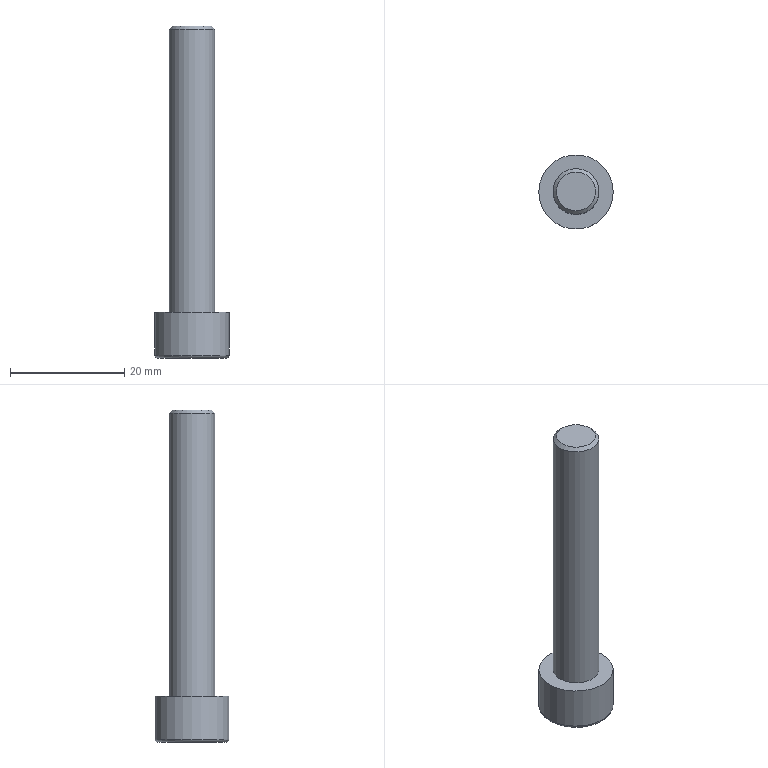Part | STEP file | 200 mesh_id82_xmt | 1 solid | 20 faces | box 13 x 13 x 58 mm | volume 3412 mm3 | plane 10 | cylinder 8 | torus 1 | cone 1 | commonest cylinder face diameters 0.6 x6 8 x1 13 x1
STEP:
#1=CARTESIAN_POINT('',(-17011.184,-4112.174,94.258));
#2=VERTEX_POINT('',#1);
#3=CARTESIAN_POINT('',(-17007.884,-4114.08,94.258));
#4=VERTEX_POINT('',#3);
#5=CARTESIAN_POINT('',(-17009.534,-4113.127,94.258));
#6=DIRECTION('',(0.866,-0.5,0.));
#7=VECTOR('',#6,1.);
#8=LINE('',#5,#7);
#9=EDGE_CURVE('',#2,#4,#8,.T.);
#10=ORIENTED_EDGE('',*,*,#9,.T.);
#11=CARTESIAN_POINT('',(-17004.584,-4112.174,94.258));
#12=VERTEX_POINT('',#11);
#13=CARTESIAN_POINT('',(-17006.234,-4113.127,94.258));
#14=DIRECTION('',(0.866,0.5,0.));
#15=VECTOR('',#14,1.);
#16=LINE('',#13,#15);
#17=EDGE_CURVE('',#4,#12,#16,.T.);
#18=ORIENTED_EDGE('',*,*,#17,.T.);
#19=CARTESIAN_POINT('',(-17004.584,-4108.364,94.258));
#20=VERTEX_POINT('',#19);
#21=CARTESIAN_POINT('',(-17004.584,-4110.269,94.258));
#22=DIRECTION('',(0.,1.,0.));
#23=VECTOR('',#22,1.);
#24=LINE('',#21,#23);
#25=EDGE_CURVE('',#12,#20,#24,.T.);
#26=ORIENTED_EDGE('',*,*,#25,.T.);
#27=CARTESIAN_POINT('',(-17007.884,-4106.459,94.258));
#28=VERTEX_POINT('',#27);
#29=CARTESIAN_POINT('',(-17006.234,-4107.411,94.258));
#30=DIRECTION('',(-0.866,0.5,0.));
#31=VECTOR('',#30,1.);
#32=LINE('',#29,#31);
#33=EDGE_CURVE('',#20,#28,#32,.T.);
#34=ORIENTED_EDGE('',*,*,#33,.T.);
#35=CARTESIAN_POINT('',(-17011.184,-4108.364,94.258));
#36=VERTEX_POINT('',#35);
#37=CARTESIAN_POINT('',(-17009.534,-4107.411,94.258));
#38=DIRECTION('',(-0.866,-0.5,0.));
#39=VECTOR('',#38,1.);
#40=LINE('',#37,#39);
#41=EDGE_CURVE('',#28,#36,#40,.T.);
#42=ORIENTED_EDGE('',*,*,#41,.T.);
#43=CARTESIAN_POINT('',(-17011.184,-4110.269,94.258));
#44=DIRECTION('',(0.,-1.,0.));
#45=VECTOR('',#44,1.);
#46=LINE('',#43,#45);
#47=EDGE_CURVE('',#36,#2,#46,.T.);
#48=ORIENTED_EDGE('',*,*,#47,.T.);
#49=EDGE_LOOP('',(#10,#18,#26,#34,#42,#48));
#50=FACE_BOUND('',#49,.T.);
#51=CARTESIAN_POINT('',(-17013.884,-4110.269,94.258));
#52=VERTEX_POINT('',#51);
#53=CARTESIAN_POINT('',(-17007.884,-4110.269,94.258));
#54=DIRECTION('',(0.,0.,-1.));
#55=DIRECTION('',(-1.,0.,0.));
#56=AXIS2_PLACEMENT_3D('',#53,#54,#55);
#57=CIRCLE('',#56,6.);
#58=EDGE_CURVE('',#52,#52,#57,.T.);
#59=ORIENTED_EDGE('',*,*,#58,.T.);
#60=EDGE_LOOP('',(#59));
#61=FACE_BOUND('',#60,.T.);
#62=CARTESIAN_POINT('',(-17007.884,-4110.269,94.258));
#63=DIRECTION('',(0.,0.,-1.));
#64=DIRECTION('',(-1.,0.,0.));
#65=AXIS2_PLACEMENT_3D('',#62,#63,#64);
#66=PLANE('',#65);
#67=ADVANCED_FACE('',(#50,#61),#66,.T.);
#68=CARTESIAN_POINT('',(-17003.884,-4110.269,151.658));
#69=VERTEX_POINT('',#68);
#70=CARTESIAN_POINT('',(-17007.884,-4110.269,151.658));
#71=DIRECTION('',(0.,0.,-1.));
#72=DIRECTION('',(1.,0.,0.));
#73=AXIS2_PLACEMENT_3D('',#70,#71,#72);
#74=CIRCLE('',#73,4.);
#75=EDGE_CURVE('',#69,#69,#74,.T.);
#76=ORIENTED_EDGE('',*,*,#75,.T.);
#77=EDGE_LOOP('',(#76));
#78=FACE_BOUND('',#77,.T.);
#79=CARTESIAN_POINT('',(-17003.884,-4110.269,102.258));
#80=VERTEX_POINT('',#79);
#81=CARTESIAN_POINT('',(-17007.884,-4110.269,102.258));
#82=DIRECTION('',(0.,0.,-1.));
#83=DIRECTION('',(1.,0.,0.));
#84=AXIS2_PLACEMENT_3D('',#81,#82,#83);
#85=CIRCLE('',#84,4.);
#86=EDGE_CURVE('',#80,#80,#85,.T.);
#87=ORIENTED_EDGE('',*,*,#86,.F.);
#88=EDGE_LOOP('',(#87));
#89=FACE_BOUND('',#88,.T.);
#90=CARTESIAN_POINT('',(-17007.884,-4110.269,102.258));
#91=DIRECTION('',(0.,0.,1.));
#92=DIRECTION('',(1.,0.,0.));
#93=AXIS2_PLACEMENT_3D('',#90,#91,#92);
#94=CYLINDRICAL_SURFACE('',#93,4.);
#95=ADVANCED_FACE('',(#78,#89),#94,.T.);
#96=ORIENTED_EDGE('',*,*,#86,.T.);
#97=EDGE_LOOP('',(#96));
#98=FACE_BOUND('',#97,.T.);
#99=CARTESIAN_POINT('',(-17001.384,-4110.269,102.258));
#100=VERTEX_POINT('',#99);
#101=CARTESIAN_POINT('',(-17007.884,-4110.269,102.258));
#102=DIRECTION('',(0.,0.,-1.));
#103=DIRECTION('',(1.,0.,0.));
#104=AXIS2_PLACEMENT_3D('',#101,#102,#103);
#105=CIRCLE('',#104,6.5);
#106=EDGE_CURVE('',#100,#100,#105,.T.);
#107=ORIENTED_EDGE('',*,*,#106,.F.);
#108=EDGE_LOOP('',(#107));
#109=FACE_BOUND('',#108,.T.);
#110=CARTESIAN_POINT('',(-17007.884,-4110.269,102.258));
#111=DIRECTION('',(0.,0.,1.));
#112=DIRECTION('',(1.,0.,0.));
#113=AXIS2_PLACEMENT_3D('',#110,#111,#112);
#114=PLANE('',#113);
#115=ADVANCED_FACE('',(#98,#109),#114,.T.);
#116=CARTESIAN_POINT('',(-17014.384,-4110.269,94.758));
#117=VERTEX_POINT('',#116);
#118=CARTESIAN_POINT('',(-17007.884,-4110.269,94.758));
#119=DIRECTION('',(0.,0.,1.));
#120=DIRECTION('',(-1.,0.,0.));
#121=AXIS2_PLACEMENT_3D('',#118,#119,#120);
#122=CIRCLE('',#121,6.5);
#123=EDGE_CURVE('',#117,#117,#122,.T.);
#124=ORIENTED_EDGE('',*,*,#123,.T.);
#125=EDGE_LOOP('',(#124));
#126=FACE_BOUND('',#125,.T.);
#127=ORIENTED_EDGE('',*,*,#106,.T.);
#128=EDGE_LOOP('',(#127));
#129=FACE_BOUND('',#128,.T.);
#130=CARTESIAN_POINT('',(-17007.884,-4110.269,102.258));
#131=DIRECTION('',(0.,0.,-1.));
#132=DIRECTION('',(1.,0.,0.));
#133=AXIS2_PLACEMENT_3D('',#130,#131,#132);
#134=CYLINDRICAL_SURFACE('',#133,6.5);
#135=ADVANCED_FACE('',(#126,#129),#134,.T.);
#136=ORIENTED_EDGE('',*,*,#58,.F.);
#137=EDGE_LOOP('',(#136));
#138=FACE_BOUND('',#137,.T.);
#139=ORIENTED_EDGE('',*,*,#123,.F.);
#140=EDGE_LOOP('',(#139));
#141=FACE_BOUND('',#140,.T.);
#142=CARTESIAN_POINT('',(-17007.884,-4110.269,94.758));
#143=DIRECTION('',(0.,0.,-1.));
#144=DIRECTION('',(-1.,0.,0.));
#145=AXIS2_PLACEMENT_3D('',#142,#143,#144);
#146=TOROIDAL_SURFACE('',#145,6.,0.5);
#147=ADVANCED_FACE('',(#138,#141),#146,.T.);
#148=CARTESIAN_POINT('',(-17007.884,-4113.733,94.558));
#149=VERTEX_POINT('',#148);
#150=CARTESIAN_POINT('',(-17007.884,-4113.733,99.258));
#151=VERTEX_POINT('',#150);
#152=CARTESIAN_POINT('',(-17007.884,-4113.733,99.258));
#153=DIRECTION('',(0.,0.,1.));
#154=VECTOR('',#153,1.);
#155=LINE('',#152,#154);
#156=EDGE_CURVE('',#149,#151,#155,.T.);
#157=ORIENTED_EDGE('',*,*,#156,.F.);
#158=CARTESIAN_POINT('',(-17010.884,-4112.001,94.558));
#159=VERTEX_POINT('',#158);
#160=CARTESIAN_POINT('',(-17010.884,-4112.001,94.558));
#161=DIRECTION('',(-0.866,0.5,0.));
#162=VECTOR('',#161,1.);
#163=LINE('',#160,#162);
#164=EDGE_CURVE('',#149,#159,#163,.T.);
#165=ORIENTED_EDGE('',*,*,#164,.T.);
#166=CARTESIAN_POINT('',(-17010.884,-4112.001,99.258));
#167=VERTEX_POINT('',#166);
#168=CARTESIAN_POINT('',(-17010.884,-4112.001,99.258));
#169=DIRECTION('',(0.,0.,1.));
#170=VECTOR('',#169,1.);
#171=LINE('',#168,#170);
#172=EDGE_CURVE('',#159,#167,#171,.T.);
#173=ORIENTED_EDGE('',*,*,#172,.T.);
#174=CARTESIAN_POINT('',(-17010.884,-4112.001,99.258));
#175=DIRECTION('',(-0.866,0.5,0.));
#176=VECTOR('',#175,1.);
#177=LINE('',#174,#176);
#178=EDGE_CURVE('',#151,#167,#177,.T.);
#179=ORIENTED_EDGE('',*,*,#178,.F.);
#180=EDGE_LOOP('',(#157,#165,#173,#179));
#181=FACE_OUTER_BOUND('',#180,.T.);
#182=CARTESIAN_POINT('',(-17010.884,-4112.001,99.258));
#183=DIRECTION('',(0.5,0.866,0.));
#184=DIRECTION('',(-0.866,0.5,0.));
#185=AXIS2_PLACEMENT_3D('',#182,#183,#184);
#186=PLANE('',#185);
#187=ADVANCED_FACE('',(#181),#186,.T.);
#188=CARTESIAN_POINT('',(-17004.884,-4112.001,94.558));
#189=VERTEX_POINT('',#188);
#190=CARTESIAN_POINT('',(-17004.884,-4112.001,99.258));
#191=VERTEX_POINT('',#190);
#192=CARTESIAN_POINT('',(-17004.884,-4112.001,99.258));
#193=DIRECTION('',(0.,0.,1.));
#194=VECTOR('',#193,1.);
#195=LINE('',#192,#194);
#196=EDGE_CURVE('',#189,#191,#195,.T.);
#197=ORIENTED_EDGE('',*,*,#196,.F.);
#198=CARTESIAN_POINT('',(-17007.884,-4113.733,94.558));
#199=DIRECTION('',(-0.866,-0.5,0.));
#200=VECTOR('',#199,1.);
#201=LINE('',#198,#200);
#202=EDGE_CURVE('',#189,#149,#201,.T.);
#203=ORIENTED_EDGE('',*,*,#202,.T.);
#204=ORIENTED_EDGE('',*,*,#156,.T.);
#205=CARTESIAN_POINT('',(-17007.884,-4113.733,99.258));
#206=DIRECTION('',(-0.866,-0.5,0.));
#207=VECTOR('',#206,1.);
#208=LINE('',#205,#207);
#209=EDGE_CURVE('',#191,#151,#208,.T.);
#210=ORIENTED_EDGE('',*,*,#209,.F.);
#211=EDGE_LOOP('',(#197,#203,#204,#210));
#212=FACE_OUTER_BOUND('',#211,.T.);
#213=CARTESIAN_POINT('',(-17007.884,-4113.733,99.258));
#214=DIRECTION('',(-0.5,0.866,0.));
#215=DIRECTION('',(-0.866,-0.5,0.));
#216=AXIS2_PLACEMENT_3D('',#213,#214,#215);
#217=PLANE('',#216);
#218=ADVANCED_FACE('',(#212),#217,.T.);
#219=CARTESIAN_POINT('',(-17004.884,-4108.537,94.558));
#220=VERTEX_POINT('',#219);
#221=CARTESIAN_POINT('',(-17004.884,-4108.537,99.258));
#222=VERTEX_POINT('',#221);
#223=CARTESIAN_POINT('',(-17004.884,-4108.537,99.258));
#224=DIRECTION('',(0.,0.,1.));
#225=VECTOR('',#224,1.);
#226=LINE('',#223,#225);
#227=EDGE_CURVE('',#220,#222,#226,.T.);
#228=ORIENTED_EDGE('',*,*,#227,.F.);
#229=CARTESIAN_POINT('',(-17004.884,-4112.001,94.558));
#230=DIRECTION('',(0.,-1.,0.));
#231=VECTOR('',#230,1.);
#232=LINE('',#229,#231);
#233=EDGE_CURVE('',#220,#189,#232,.T.);
#234=ORIENTED_EDGE('',*,*,#233,.T.);
#235=ORIENTED_EDGE('',*,*,#196,.T.);
#236=CARTESIAN_POINT('',(-17004.884,-4112.001,99.258));
#237=DIRECTION('',(0.,-1.,0.));
#238=VECTOR('',#237,1.);
#239=LINE('',#236,#238);
#240=EDGE_CURVE('',#222,#191,#239,.T.);
#241=ORIENTED_EDGE('',*,*,#240,.F.);
#242=EDGE_LOOP('',(#228,#234,#235,#241));
#243=FACE_OUTER_BOUND('',#242,.T.);
#244=CARTESIAN_POINT('',(-17004.884,-4112.001,99.258));
#245=DIRECTION('',(-1.,0.,0.));
#246=DIRECTION('',(0.,0.,1.));
#247=AXIS2_PLACEMENT_3D('',#244,#245,#246);
#248=PLANE('',#247);
#249=ADVANCED_FACE('',(#243),#248,.T.);
#250=CARTESIAN_POINT('',(-17007.884,-4106.805,94.558));
#251=VERTEX_POINT('',#250);
#252=CARTESIAN_POINT('',(-17007.884,-4106.805,99.258));
#253=VERTEX_POINT('',#252);
#254=CARTESIAN_POINT('',(-17007.884,-4106.805,99.258));
#255=DIRECTION('',(0.,0.,1.));
#256=VECTOR('',#255,1.);
#257=LINE('',#254,#256);
#258=EDGE_CURVE('',#251,#253,#257,.T.);
#259=ORIENTED_EDGE('',*,*,#258,.F.);
#260=CARTESIAN_POINT('',(-17004.884,-4108.537,94.558));
#261=DIRECTION('',(0.866,-0.5,0.));
#262=VECTOR('',#261,1.);
#263=LINE('',#260,#262);
#264=EDGE_CURVE('',#251,#220,#263,.T.);
#265=ORIENTED_EDGE('',*,*,#264,.T.);
#266=ORIENTED_EDGE('',*,*,#227,.T.);
#267=CARTESIAN_POINT('',(-17004.884,-4108.537,99.258));
#268=DIRECTION('',(0.866,-0.5,0.));
#269=VECTOR('',#268,1.);
#270=LINE('',#267,#269);
#271=EDGE_CURVE('',#253,#222,#270,.T.);
#272=ORIENTED_EDGE('',*,*,#271,.F.);
#273=EDGE_LOOP('',(#259,#265,#266,#272));
#274=FACE_OUTER_BOUND('',#273,.T.);
#275=CARTESIAN_POINT('',(-17004.884,-4108.537,99.258));
#276=DIRECTION('',(-0.5,-0.866,0.));
#277=DIRECTION('',(0.866,-0.5,0.));
#278=AXIS2_PLACEMENT_3D('',#275,#276,#277);
#279=PLANE('',#278);
#280=ADVANCED_FACE('',(#274),#279,.T.);
#281=CARTESIAN_POINT('',(-17010.884,-4108.537,94.558));
#282=VERTEX_POINT('',#281);
#283=CARTESIAN_POINT('',(-17010.884,-4108.537,99.258));
#284=VERTEX_POINT('',#283);
#285=CARTESIAN_POINT('',(-17010.884,-4108.537,99.258));
#286=DIRECTION('',(0.,0.,1.));
#287=VECTOR('',#286,1.);
#288=LINE('',#285,#287);
#289=EDGE_CURVE('',#282,#284,#288,.T.);
#290=ORIENTED_EDGE('',*,*,#289,.F.);
#291=CARTESIAN_POINT('',(-17007.884,-4106.805,94.558));
#292=DIRECTION('',(0.866,0.5,0.));
#293=VECTOR('',#292,1.);
#294=LINE('',#291,#293);
#295=EDGE_CURVE('',#282,#251,#294,.T.);
#296=ORIENTED_EDGE('',*,*,#295,.T.);
#297=ORIENTED_EDGE('',*,*,#258,.T.);
#298=CARTESIAN_POINT('',(-17007.884,-4106.805,99.258));
#299=DIRECTION('',(0.866,0.5,0.));
#300=VECTOR('',#299,1.);
#301=LINE('',#298,#300);
#302=EDGE_CURVE('',#284,#253,#301,.T.);
#303=ORIENTED_EDGE('',*,*,#302,.F.);
#304=EDGE_LOOP('',(#290,#296,#297,#303));
#305=FACE_OUTER_BOUND('',#304,.T.);
#306=CARTESIAN_POINT('',(-17007.884,-4106.805,99.258));
#307=DIRECTION('',(0.5,-0.866,0.));
#308=DIRECTION('',(0.866,0.5,0.));
#309=AXIS2_PLACEMENT_3D('',#306,#307,#308);
#310=PLANE('',#309);
#311=ADVANCED_FACE('',(#305),#310,.T.);
#312=ORIENTED_EDGE('',*,*,#172,.F.);
#313=CARTESIAN_POINT('',(-17010.884,-4108.537,94.558));
#314=DIRECTION('',(0.,1.,0.));
#315=VECTOR('',#314,1.);
#316=LINE('',#313,#315);
#317=EDGE_CURVE('',#159,#282,#316,.T.);
#318=ORIENTED_EDGE('',*,*,#317,.T.);
#319=ORIENTED_EDGE('',*,*,#289,.T.);
#320=CARTESIAN_POINT('',(-17010.884,-4108.537,99.258));
#321=DIRECTION('',(0.,1.,0.));
#322=VECTOR('',#321,1.);
#323=LINE('',#320,#322);
#324=EDGE_CURVE('',#167,#284,#323,.T.);
#325=ORIENTED_EDGE('',*,*,#324,.F.);
#326=EDGE_LOOP('',(#312,#318,#319,#325));
#327=FACE_OUTER_BOUND('',#326,.T.);
#328=CARTESIAN_POINT('',(-17010.884,-4108.537,99.258));
#329=DIRECTION('',(1.,0.,0.));
#330=DIRECTION('',(0.,0.,-1.));
#331=AXIS2_PLACEMENT_3D('',#328,#329,#330);
#332=PLANE('',#331);
#333=ADVANCED_FACE('',(#327),#332,.T.);
#334=ORIENTED_EDGE('',*,*,#178,.T.);
#335=ORIENTED_EDGE('',*,*,#324,.T.);
#336=ORIENTED_EDGE('',*,*,#302,.T.);
#337=ORIENTED_EDGE('',*,*,#271,.T.);
#338=ORIENTED_EDGE('',*,*,#240,.T.);
#339=ORIENTED_EDGE('',*,*,#209,.T.);
#340=EDGE_LOOP('',(#334,#335,#336,#337,#338,#339));
#341=FACE_OUTER_BOUND('',#340,.T.);
#342=CARTESIAN_POINT('',(0.,-5.,99.258));
#343=DIRECTION('',(0.,0.,1.));
#344=DIRECTION('',(1.,0.,0.));
#345=AXIS2_PLACEMENT_3D('',#342,#343,#344);
#346=PLANE('',#345);
#347=ADVANCED_FACE('',(#341),#346,.F.);
#348=CARTESIAN_POINT('',(-17007.884,-4106.459,94.558));
#349=DIRECTION('',(1.,0.,0.));
#350=DIRECTION('',(0.,1.,0.));
#351=AXIS2_PLACEMENT_3D('',#348,#349,#350);
#352=ELLIPSE('',#351,0.3464,0.3);
#353=EDGE_CURVE('',#251,#28,#352,.T.);
#354=ORIENTED_EDGE('',*,*,#353,.F.);
#355=ORIENTED_EDGE('',*,*,#295,.F.);
#356=CARTESIAN_POINT('',(-17011.184,-4108.364,94.558));
#357=DIRECTION('',(-0.5,-0.866,0.));
#358=DIRECTION('',(-0.866,0.5,0.));
#359=AXIS2_PLACEMENT_3D('',#356,#357,#358);
#360=ELLIPSE('',#359,0.3464,0.3);
#361=EDGE_CURVE('',#36,#282,#360,.T.);
#362=ORIENTED_EDGE('',*,*,#361,.F.);
#363=ORIENTED_EDGE('',*,*,#41,.F.);
#364=EDGE_LOOP('',(#354,#355,#362,#363));
#365=FACE_OUTER_BOUND('',#364,.T.);
#366=CARTESIAN_POINT('',(-17009.534,-4107.411,94.558));
#367=DIRECTION('',(-0.866,-0.5,0.));
#368=DIRECTION('',(0.5,-0.866,0.));
#369=AXIS2_PLACEMENT_3D('',#366,#367,#368);
#370=CYLINDRICAL_SURFACE('',#369,0.3);
#371=ADVANCED_FACE('',(#365),#370,.T.);
#372=ORIENTED_EDGE('',*,*,#361,.T.);
#373=ORIENTED_EDGE('',*,*,#317,.F.);
#374=CARTESIAN_POINT('',(-17011.184,-4112.174,94.558));
#375=DIRECTION('',(0.5,-0.866,0.));
#376=DIRECTION('',(-0.866,-0.5,0.));
#377=AXIS2_PLACEMENT_3D('',#374,#375,#376);
#378=ELLIPSE('',#377,0.3464,0.3);
#379=EDGE_CURVE('',#2,#159,#378,.T.);
#380=ORIENTED_EDGE('',*,*,#379,.F.);
#381=ORIENTED_EDGE('',*,*,#47,.F.);
#382=EDGE_LOOP('',(#372,#373,#380,#381));
#383=FACE_OUTER_BOUND('',#382,.T.);
#384=CARTESIAN_POINT('',(-17011.184,-4110.269,94.558));
#385=DIRECTION('',(0.,-1.,0.));
#386=DIRECTION('',(0.,0.,-1.));
#387=AXIS2_PLACEMENT_3D('',#384,#385,#386);
#388=CYLINDRICAL_SURFACE('',#387,0.3);
#389=ADVANCED_FACE('',(#383),#388,.T.);
#390=ORIENTED_EDGE('',*,*,#353,.T.);
#391=ORIENTED_EDGE('',*,*,#33,.F.);
#392=CARTESIAN_POINT('',(-17004.584,-4108.364,94.558));
#393=DIRECTION('',(0.5,-0.866,0.));
#394=DIRECTION('',(0.866,0.5,0.));
#395=AXIS2_PLACEMENT_3D('',#392,#393,#394);
#396=ELLIPSE('',#395,0.3464,0.3);
#397=EDGE_CURVE('',#220,#20,#396,.T.);
#398=ORIENTED_EDGE('',*,*,#397,.F.);
#399=ORIENTED_EDGE('',*,*,#264,.F.);
#400=EDGE_LOOP('',(#390,#391,#398,#399));
#401=FACE_OUTER_BOUND('',#400,.T.);
#402=CARTESIAN_POINT('',(-17006.234,-4107.411,94.558));
#403=DIRECTION('',(-0.866,0.5,0.));
#404=DIRECTION('',(-0.5,-0.866,0.));
#405=AXIS2_PLACEMENT_3D('',#402,#403,#404);
#406=CYLINDRICAL_SURFACE('',#405,0.3);
#407=ADVANCED_FACE('',(#401),#406,.T.);
#408=ORIENTED_EDGE('',*,*,#379,.T.);
#409=ORIENTED_EDGE('',*,*,#164,.F.);
#410=CARTESIAN_POINT('',(-17007.884,-4114.08,94.558));
#411=DIRECTION('',(1.,0.,0.));
#412=DIRECTION('',(0.,1.,0.));
#413=AXIS2_PLACEMENT_3D('',#410,#411,#412);
#414=ELLIPSE('',#413,0.3464,0.3);
#415=EDGE_CURVE('',#4,#149,#414,.T.);
#416=ORIENTED_EDGE('',*,*,#415,.F.);
#417=ORIENTED_EDGE('',*,*,#9,.F.);
#418=EDGE_LOOP('',(#408,#409,#416,#417));
#419=FACE_OUTER_BOUND('',#418,.T.);
#420=CARTESIAN_POINT('',(-17009.534,-4113.127,94.558));
#421=DIRECTION('',(0.866,-0.5,0.));
#422=DIRECTION('',(0.5,0.866,0.));
#423=AXIS2_PLACEMENT_3D('',#420,#421,#422);
#424=CYLINDRICAL_SURFACE('',#423,0.3);
#425=ADVANCED_FACE('',(#419),#424,.T.);
#426=ORIENTED_EDGE('',*,*,#397,.T.);
#427=ORIENTED_EDGE('',*,*,#25,.F.);
#428=CARTESIAN_POINT('',(-17004.584,-4112.174,94.558));
#429=DIRECTION('',(-0.5,-0.866,0.));
#430=DIRECTION('',(0.866,-0.5,0.));
#431=AXIS2_PLACEMENT_3D('',#428,#429,#430);
#432=ELLIPSE('',#431,0.3464,0.3);
#433=EDGE_CURVE('',#189,#12,#432,.T.);
#434=ORIENTED_EDGE('',*,*,#433,.F.);
#435=ORIENTED_EDGE('',*,*,#233,.F.);
#436=EDGE_LOOP('',(#426,#427,#434,#435));
#437=FACE_OUTER_BOUND('',#436,.T.);
#438=CARTESIAN_POINT('',(-17004.584,-4110.269,94.558));
#439=DIRECTION('',(0.,1.,0.));
#440=DIRECTION('',(0.,0.,1.));
#441=AXIS2_PLACEMENT_3D('',#438,#439,#440);
#442=CYLINDRICAL_SURFACE('',#441,0.3);
#443=ADVANCED_FACE('',(#437),#442,.T.);
#444=ORIENTED_EDGE('',*,*,#415,.T.);
#445=ORIENTED_EDGE('',*,*,#202,.F.);
#446=ORIENTED_EDGE('',*,*,#433,.T.);
#447=ORIENTED_EDGE('',*,*,#17,.F.);
#448=EDGE_LOOP('',(#444,#445,#446,#447));
#449=FACE_OUTER_BOUND('',#448,.T.);
#450=CARTESIAN_POINT('',(-17006.234,-4113.127,94.558));
#451=DIRECTION('',(0.866,0.5,0.));
#452=DIRECTION('',(-0.5,0.866,0.));
#453=AXIS2_PLACEMENT_3D('',#450,#451,#452);
#454=CYLINDRICAL_SURFACE('',#453,0.3);
#455=ADVANCED_FACE('',(#449),#454,.T.);
#456=CARTESIAN_POINT('',(-17004.484,-4110.269,152.258));
#457=VERTEX_POINT('',#456);
#458=CARTESIAN_POINT('',(-17007.884,-4110.269,152.258));
#459=DIRECTION('',(0.,0.,1.));
#460=DIRECTION('',(1.,0.,0.));
#461=AXIS2_PLACEMENT_3D('',#458,#459,#460);
#462=CIRCLE('',#461,3.4);
#463=EDGE_CURVE('',#457,#457,#462,.T.);
#464=ORIENTED_EDGE('',*,*,#463,.T.);
#465=EDGE_LOOP('',(#464));
#466=FACE_OUTER_BOUND('',#465,.T.);
#467=CARTESIAN_POINT('',(-17007.884,-4110.269,152.258));
#468=DIRECTION('',(0.,0.,1.));
#469=DIRECTION('',(1.,0.,0.));
#470=AXIS2_PLACEMENT_3D('',#467,#468,#469);
#471=PLANE('',#470);
#472=ADVANCED_FACE('',(#466),#471,.T.);
#473=ORIENTED_EDGE('',*,*,#463,.F.);
#474=EDGE_LOOP('',(#473));
#475=FACE_BOUND('',#474,.T.);
#476=ORIENTED_EDGE('',*,*,#75,.F.);
#477=EDGE_LOOP('',(#476));
#478=FACE_BOUND('',#477,.T.);
#479=CARTESIAN_POINT('',(-17007.884,-4110.269,151.658));
#480=DIRECTION('',(0.,0.,-1.));
#481=DIRECTION('',(-1.,0.,0.));
#482=AXIS2_PLACEMENT_3D('',#479,#480,#481);
#483=CONICAL_SURFACE('',#482,4.,45.);
#484=ADVANCED_FACE('',(#475,#478),#483,.T.);
#485=CLOSED_SHELL('',(#67,#95,#115,#135,#147,#187,#218,#249,#280,#311,#333,#347,#371,#389,#407,#425,#443,#455,#472,#484));
#486=MANIFOLD_SOLID_BREP('',#485);
#487=(LENGTH_UNIT()NAMED_UNIT(*)SI_UNIT(.MILLI.,.METRE.));
#488=UNCERTAINTY_MEASURE_WITH_UNIT(LENGTH_MEASURE(0.00002),#487,'','');
#489=(NAMED_UNIT(*)PLANE_ANGLE_UNIT()SI_UNIT($,.RADIAN.));
#490=PLANE_ANGLE_MEASURE_WITH_UNIT(PLANE_ANGLE_MEASURE(0.01745),#489);
#491=DIMENSIONAL_EXPONENTS(0.,0.,0.,0.,0.,0.,0.);
#492=(CONVERSION_BASED_UNIT('DEGREE',#490)NAMED_UNIT(#491)PLANE_ANGLE_UNIT());
#493=(NAMED_UNIT(*)SI_UNIT($,.STERADIAN.)SOLID_ANGLE_UNIT());
#494=(GEOMETRIC_REPRESENTATION_CONTEXT(3)GLOBAL_UNCERTAINTY_ASSIGNED_CONTEXT((#488))GLOBAL_UNIT_ASSIGNED_CONTEXT((#487,#492,#493))REPRESENTATION_CONTEXT('',''));
#495=ADVANCED_BREP_SHAPE_REPRESENTATION('',(#486),#494);